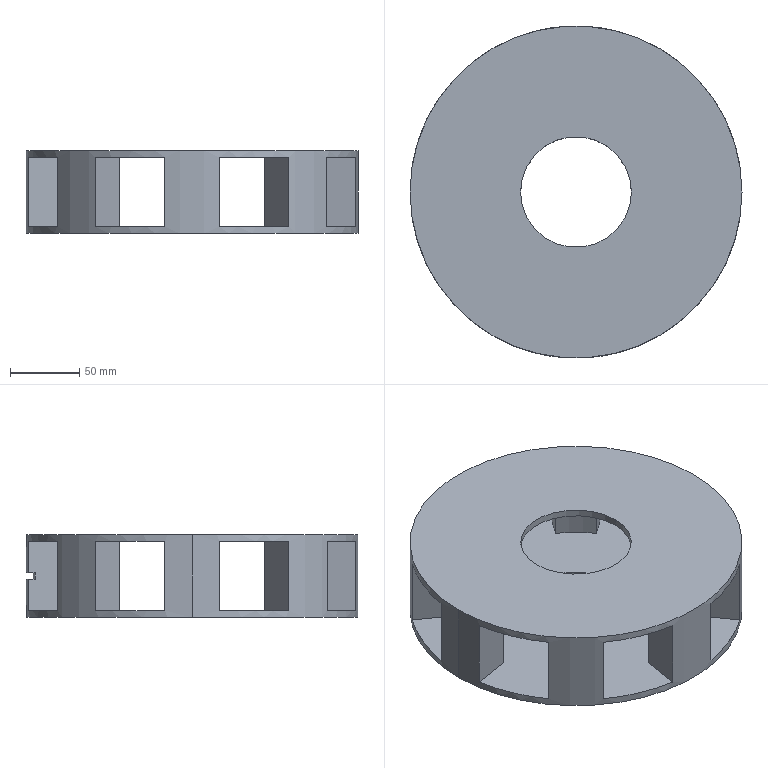Part | SolidWorks | features ICE 6, CirPattern 2, Extrusion 1, RevCut 1 | 1 solid | 38 faces | box 240 x 240 x 59.97 mm | volume 814702 mm3 | plane 22 | cylinder 16 | commonest cylinder face diameters 180 x9 80.06 x4 240 x2 230 x1
STEP:
#1=CARTESIAN_POINT('',(40.03,0.,5.));
#2=VERTEX_POINT('',#1);
#3=CARTESIAN_POINT('',(-40.03,0.,5.));
#4=VERTEX_POINT('',#3);
#5=CARTESIAN_POINT('',(0.,0.,5.));
#6=DIRECTION('',(0.,0.,-1.));
#7=DIRECTION('',(-1.,0.,0.));
#8=AXIS2_PLACEMENT_3D('',#5,#6,#7);
#9=CIRCLE('',#8,40.03);
#10=EDGE_CURVE('',#2,#4,#9,.T.);
#11=ORIENTED_EDGE('',*,*,#10,.F.);
#12=CARTESIAN_POINT('',(40.03,0.,0.));
#13=VERTEX_POINT('',#12);
#14=CARTESIAN_POINT('',(40.03,0.,5.));
#15=DIRECTION('',(0.,0.,-1.));
#16=VECTOR('',#15,1000.);
#17=LINE('',#14,#16);
#18=EDGE_CURVE('',#2,#13,#17,.T.);
#19=ORIENTED_EDGE('',*,*,#18,.T.);
#20=CARTESIAN_POINT('',(-40.03,0.,0.));
#21=VERTEX_POINT('',#20);
#22=CARTESIAN_POINT('',(0.,0.,0.));
#23=DIRECTION('',(0.,0.,-1.));
#24=DIRECTION('',(-1.,0.,0.));
#25=AXIS2_PLACEMENT_3D('',#22,#23,#24);
#26=CIRCLE('',#25,40.03);
#27=EDGE_CURVE('',#13,#21,#26,.T.);
#28=ORIENTED_EDGE('',*,*,#27,.T.);
#29=CARTESIAN_POINT('',(-40.03,0.,5.));
#30=DIRECTION('',(0.,0.,-1.));
#31=VECTOR('',#30,1000.);
#32=LINE('',#29,#31);
#33=EDGE_CURVE('',#4,#21,#32,.T.);
#34=ORIENTED_EDGE('',*,*,#33,.F.);
#35=EDGE_LOOP('',(#11,#19,#28,#34));
#36=FACE_OUTER_BOUND('',#35,.T.);
#37=CARTESIAN_POINT('',(0.,0.,5.));
#38=DIRECTION('',(0.,0.,-1.));
#39=DIRECTION('',(-1.,0.,0.));
#40=AXIS2_PLACEMENT_3D('',#37,#38,#39);
#41=CYLINDRICAL_SURFACE('',#40,40.03);
#42=ADVANCED_FACE('',(#36),#41,.F.);
#43=CARTESIAN_POINT('',(-40.03,0.,54.97));
#44=VERTEX_POINT('',#43);
#45=CARTESIAN_POINT('',(40.03,0.,54.97));
#46=VERTEX_POINT('',#45);
#47=CARTESIAN_POINT('',(0.,0.,54.97));
#48=DIRECTION('',(0.,0.,1.));
#49=DIRECTION('',(1.,0.,0.));
#50=AXIS2_PLACEMENT_3D('',#47,#48,#49);
#51=CIRCLE('',#50,40.03);
#52=EDGE_CURVE('',#44,#46,#51,.T.);
#53=ORIENTED_EDGE('',*,*,#52,.F.);
#54=CARTESIAN_POINT('',(-40.03,0.,59.97));
#55=VERTEX_POINT('',#54);
#56=CARTESIAN_POINT('',(-40.03,0.,54.97));
#57=DIRECTION('',(0.,0.,1.));
#58=VECTOR('',#57,1000.);
#59=LINE('',#56,#58);
#60=EDGE_CURVE('',#44,#55,#59,.T.);
#61=ORIENTED_EDGE('',*,*,#60,.T.);
#62=CARTESIAN_POINT('',(40.03,0.,59.97));
#63=VERTEX_POINT('',#62);
#64=CARTESIAN_POINT('',(0.,0.,59.97));
#65=DIRECTION('',(0.,0.,1.));
#66=DIRECTION('',(1.,0.,0.));
#67=AXIS2_PLACEMENT_3D('',#64,#65,#66);
#68=CIRCLE('',#67,40.03);
#69=EDGE_CURVE('',#55,#63,#68,.T.);
#70=ORIENTED_EDGE('',*,*,#69,.T.);
#71=CARTESIAN_POINT('',(40.03,0.,54.97));
#72=DIRECTION('',(0.,0.,1.));
#73=VECTOR('',#72,1000.);
#74=LINE('',#71,#73);
#75=EDGE_CURVE('',#46,#63,#74,.T.);
#76=ORIENTED_EDGE('',*,*,#75,.F.);
#77=EDGE_LOOP('',(#53,#61,#70,#76));
#78=FACE_OUTER_BOUND('',#77,.T.);
#79=CARTESIAN_POINT('',(0.,0.,54.97));
#80=DIRECTION('',(0.,0.,1.));
#81=DIRECTION('',(1.,0.,0.));
#82=AXIS2_PLACEMENT_3D('',#79,#80,#81);
#83=CYLINDRICAL_SURFACE('',#82,40.03);
#84=ADVANCED_FACE('',(#78),#83,.F.);
#85=CARTESIAN_POINT('',(-19.619,118.385,5.));
#86=VERTEX_POINT('',#85);
#87=CARTESIAN_POINT('',(-19.619,118.385,27.485));
#88=VERTEX_POINT('',#87);
#89=CARTESIAN_POINT('',(-19.619,118.385,80.));
#90=DIRECTION('',(0.,0.,1.));
#91=VECTOR('',#90,1000.);
#92=LINE('',#89,#91);
#93=EDGE_CURVE('',#86,#88,#92,.T.);
#94=ORIENTED_EDGE('',*,*,#93,.T.);
#95=CARTESIAN_POINT('',(19.619,118.385,27.485));
#96=VERTEX_POINT('',#95);
#97=CARTESIAN_POINT('',(0.,0.,27.485));
#98=DIRECTION('',(0.,0.,-1.));
#99=DIRECTION('',(-1.,0.,0.));
#100=AXIS2_PLACEMENT_3D('',#97,#98,#99);
#101=CIRCLE('',#100,120.);
#102=EDGE_CURVE('',#88,#96,#101,.T.);
#103=ORIENTED_EDGE('',*,*,#102,.T.);
#104=CARTESIAN_POINT('',(19.619,118.385,5.));
#105=VERTEX_POINT('',#104);
#106=CARTESIAN_POINT('',(19.619,118.385,80.));
#107=DIRECTION('',(0.,0.,-1.));
#108=VECTOR('',#107,1000.);
#109=LINE('',#106,#108);
#110=EDGE_CURVE('',#96,#105,#109,.T.);
#111=ORIENTED_EDGE('',*,*,#110,.T.);
#112=CARTESIAN_POINT('',(69.838,97.584,5.));
#113=VERTEX_POINT('',#112);
#114=CARTESIAN_POINT('',(0.,0.,5.));
#115=DIRECTION('',(0.,0.,-1.));
#116=DIRECTION('',(-1.,0.,0.));
#117=AXIS2_PLACEMENT_3D('',#114,#115,#116);
#118=CIRCLE('',#117,120.);
#119=EDGE_CURVE('',#105,#113,#118,.T.);
#120=ORIENTED_EDGE('',*,*,#119,.T.);
#121=CARTESIAN_POINT('',(69.838,97.584,54.97));
#122=VERTEX_POINT('',#121);
#123=CARTESIAN_POINT('',(69.838,97.584,80.));
#124=DIRECTION('',(0.,0.,1.));
#125=VECTOR('',#124,1000.);
#126=LINE('',#123,#125);
#127=EDGE_CURVE('',#113,#122,#126,.T.);
#128=ORIENTED_EDGE('',*,*,#127,.T.);
#129=CARTESIAN_POINT('',(19.619,118.385,54.97));
#130=VERTEX_POINT('',#129);
#131=CARTESIAN_POINT('',(0.,0.,54.97));
#132=DIRECTION('',(0.,0.,-1.));
#133=DIRECTION('',(-1.,0.,0.));
#134=AXIS2_PLACEMENT_3D('',#131,#132,#133);
#135=CIRCLE('',#134,120.);
#136=EDGE_CURVE('',#130,#122,#135,.T.);
#137=ORIENTED_EDGE('',*,*,#136,.F.);
#138=CARTESIAN_POINT('',(19.619,118.385,32.485));
#139=VERTEX_POINT('',#138);
#140=CARTESIAN_POINT('',(19.619,118.385,80.));
#141=DIRECTION('',(0.,0.,-1.));
#142=VECTOR('',#141,1000.);
#143=LINE('',#140,#142);
#144=EDGE_CURVE('',#130,#139,#143,.T.);
#145=ORIENTED_EDGE('',*,*,#144,.T.);
#146=CARTESIAN_POINT('',(-19.619,118.385,32.485));
#147=VERTEX_POINT('',#146);
#148=CARTESIAN_POINT('',(0.,0.,32.485));
#149=DIRECTION('',(0.,0.,1.));
#150=DIRECTION('',(1.,0.,0.));
#151=AXIS2_PLACEMENT_3D('',#148,#149,#150);
#152=CIRCLE('',#151,120.);
#153=EDGE_CURVE('',#139,#147,#152,.T.);
#154=ORIENTED_EDGE('',*,*,#153,.T.);
#155=CARTESIAN_POINT('',(-19.619,118.385,54.97));
#156=VERTEX_POINT('',#155);
#157=CARTESIAN_POINT('',(-19.619,118.385,80.));
#158=DIRECTION('',(0.,0.,1.));
#159=VECTOR('',#158,1000.);
#160=LINE('',#157,#159);
#161=EDGE_CURVE('',#147,#156,#160,.T.);
#162=ORIENTED_EDGE('',*,*,#161,.T.);
#163=CARTESIAN_POINT('',(-69.838,97.584,54.97));
#164=VERTEX_POINT('',#163);
#165=CARTESIAN_POINT('',(0.,0.,54.97));
#166=DIRECTION('',(0.,0.,-1.));
#167=DIRECTION('',(-1.,0.,0.));
#168=AXIS2_PLACEMENT_3D('',#165,#166,#167);
#169=CIRCLE('',#168,120.);
#170=EDGE_CURVE('',#164,#156,#169,.T.);
#171=ORIENTED_EDGE('',*,*,#170,.F.);
#172=CARTESIAN_POINT('',(-69.838,97.584,5.));
#173=VERTEX_POINT('',#172);
#174=CARTESIAN_POINT('',(-69.838,97.584,80.));
#175=DIRECTION('',(0.,0.,-1.));
#176=VECTOR('',#175,1000.);
#177=LINE('',#174,#176);
#178=EDGE_CURVE('',#164,#173,#177,.T.);
#179=ORIENTED_EDGE('',*,*,#178,.T.);
#180=CARTESIAN_POINT('',(0.,0.,5.));
#181=DIRECTION('',(0.,0.,-1.));
#182=DIRECTION('',(-1.,0.,0.));
#183=AXIS2_PLACEMENT_3D('',#180,#181,#182);
#184=CIRCLE('',#183,120.);
#185=EDGE_CURVE('',#173,#86,#184,.T.);
#186=ORIENTED_EDGE('',*,*,#185,.T.);
#187=EDGE_LOOP('',(#94,#103,#111,#120,#128,#137,#145,#154,#162,#171,#179,#186));
#188=FACE_BOUND('',#187,.T.);
#189=CARTESIAN_POINT('',(97.584,69.838,54.97));
#190=VERTEX_POINT('',#189);
#191=CARTESIAN_POINT('',(97.584,69.838,5.));
#192=VERTEX_POINT('',#191);
#193=CARTESIAN_POINT('',(97.584,69.838,80.));
#194=DIRECTION('',(0.,0.,-1.));
#195=VECTOR('',#194,1000.);
#196=LINE('',#193,#195);
#197=EDGE_CURVE('',#190,#192,#196,.T.);
#198=ORIENTED_EDGE('',*,*,#197,.T.);
#199=CARTESIAN_POINT('',(118.385,19.619,5.));
#200=VERTEX_POINT('',#199);
#201=CARTESIAN_POINT('',(0.,0.,5.));
#202=DIRECTION('',(0.,0.,-1.));
#203=DIRECTION('',(-1.,0.,0.));
#204=AXIS2_PLACEMENT_3D('',#201,#202,#203);
#205=CIRCLE('',#204,120.);
#206=EDGE_CURVE('',#192,#200,#205,.T.);
#207=ORIENTED_EDGE('',*,*,#206,.T.);
#208=CARTESIAN_POINT('',(118.385,19.619,54.97));
#209=VERTEX_POINT('',#208);
#210=CARTESIAN_POINT('',(118.385,19.619,80.));
#211=DIRECTION('',(0.,0.,1.));
#212=VECTOR('',#211,1000.);
#213=LINE('',#210,#212);
#214=EDGE_CURVE('',#200,#209,#213,.T.);
#215=ORIENTED_EDGE('',*,*,#214,.T.);
#216=CARTESIAN_POINT('',(0.,0.,54.97));
#217=DIRECTION('',(0.,0.,-1.));
#218=DIRECTION('',(-1.,0.,0.));
#219=AXIS2_PLACEMENT_3D('',#216,#217,#218);
#220=CIRCLE('',#219,120.);
#221=EDGE_CURVE('',#190,#209,#220,.T.);
#222=ORIENTED_EDGE('',*,*,#221,.F.);
#223=EDGE_LOOP('',(#198,#207,#215,#222));
#224=FACE_BOUND('',#223,.T.);
#225=CARTESIAN_POINT('',(-118.385,19.619,54.97));
#226=VERTEX_POINT('',#225);
#227=CARTESIAN_POINT('',(-118.385,19.619,5.));
#228=VERTEX_POINT('',#227);
#229=CARTESIAN_POINT('',(-118.385,19.619,80.));
#230=DIRECTION('',(0.,0.,-1.));
#231=VECTOR('',#230,1000.);
#232=LINE('',#229,#231);
#233=EDGE_CURVE('',#226,#228,#232,.T.);
#234=ORIENTED_EDGE('',*,*,#233,.T.);
#235=CARTESIAN_POINT('',(-97.584,69.838,5.));
#236=VERTEX_POINT('',#235);
#237=CARTESIAN_POINT('',(0.,0.,5.));
#238=DIRECTION('',(0.,0.,-1.));
#239=DIRECTION('',(-1.,0.,0.));
#240=AXIS2_PLACEMENT_3D('',#237,#238,#239);
#241=CIRCLE('',#240,120.);
#242=EDGE_CURVE('',#228,#236,#241,.T.);
#243=ORIENTED_EDGE('',*,*,#242,.T.);
#244=CARTESIAN_POINT('',(-97.584,69.838,54.97));
#245=VERTEX_POINT('',#244);
#246=CARTESIAN_POINT('',(-97.584,69.838,80.));
#247=DIRECTION('',(0.,0.,1.));
#248=VECTOR('',#247,1000.);
#249=LINE('',#246,#248);
#250=EDGE_CURVE('',#236,#245,#249,.T.);
#251=ORIENTED_EDGE('',*,*,#250,.T.);
#252=CARTESIAN_POINT('',(0.,0.,54.97));
#253=DIRECTION('',(0.,0.,-1.));
#254=DIRECTION('',(-1.,0.,0.));
#255=AXIS2_PLACEMENT_3D('',#252,#253,#254);
#256=CIRCLE('',#255,120.);
#257=EDGE_CURVE('',#226,#245,#256,.T.);
#258=ORIENTED_EDGE('',*,*,#257,.F.);
#259=EDGE_LOOP('',(#234,#243,#251,#258));
#260=FACE_BOUND('',#259,.T.);
#261=CARTESIAN_POINT('',(-120.,0.,0.));
#262=VERTEX_POINT('',#261);
#263=CARTESIAN_POINT('',(120.,0.,0.));
#264=VERTEX_POINT('',#263);
#265=CARTESIAN_POINT('',(0.,0.,0.));
#266=DIRECTION('',(0.,0.,-1.));
#267=DIRECTION('',(1.,0.,0.));
#268=AXIS2_PLACEMENT_3D('',#265,#266,#267);
#269=CIRCLE('',#268,120.);
#270=EDGE_CURVE('',#262,#264,#269,.T.);
#271=ORIENTED_EDGE('',*,*,#270,.F.);
#272=CARTESIAN_POINT('',(-120.,0.,59.97));
#273=VERTEX_POINT('',#272);
#274=CARTESIAN_POINT('',(-120.,0.,0.));
#275=DIRECTION('',(0.,0.,1.));
#276=VECTOR('',#275,1000.);
#277=LINE('',#274,#276);
#278=EDGE_CURVE('',#262,#273,#277,.T.);
#279=ORIENTED_EDGE('',*,*,#278,.T.);
#280=CARTESIAN_POINT('',(120.,0.,59.97));
#281=VERTEX_POINT('',#280);
#282=CARTESIAN_POINT('',(0.,0.,59.97));
#283=DIRECTION('',(0.,0.,-1.));
#284=DIRECTION('',(1.,0.,0.));
#285=AXIS2_PLACEMENT_3D('',#282,#283,#284);
#286=CIRCLE('',#285,120.);
#287=EDGE_CURVE('',#273,#281,#286,.T.);
#288=ORIENTED_EDGE('',*,*,#287,.T.);
#289=CARTESIAN_POINT('',(120.,0.,0.));
#290=DIRECTION('',(0.,0.,1.));
#291=VECTOR('',#290,1000.);
#292=LINE('',#289,#291);
#293=EDGE_CURVE('',#264,#281,#292,.T.);
#294=ORIENTED_EDGE('',*,*,#293,.F.);
#295=EDGE_LOOP('',(#271,#279,#288,#294));
#296=FACE_OUTER_BOUND('',#295,.T.);
#297=CARTESIAN_POINT('',(0.,0.,0.));
#298=DIRECTION('',(0.,0.,1.));
#299=DIRECTION('',(1.,0.,0.));
#300=AXIS2_PLACEMENT_3D('',#297,#298,#299);
#301=CYLINDRICAL_SURFACE('',#300,120.);
#302=ADVANCED_FACE('',(#188,#224,#260,#296),#301,.T.);
#303=CARTESIAN_POINT('',(88.789,14.715,5.));
#304=VERTEX_POINT('',#303);
#305=CARTESIAN_POINT('',(90.,0.,5.));
#306=VERTEX_POINT('',#305);
#307=CARTESIAN_POINT('',(0.,0.,5.));
#308=DIRECTION('',(0.,0.,-1.));
#309=DIRECTION('',(-1.,0.,0.));
#310=AXIS2_PLACEMENT_3D('',#307,#308,#309);
#311=CIRCLE('',#310,90.);
#312=EDGE_CURVE('',#304,#306,#311,.T.);
#313=ORIENTED_EDGE('',*,*,#312,.T.);
#314=CARTESIAN_POINT('',(90.,0.,54.97));
#315=VERTEX_POINT('',#314);
#316=CARTESIAN_POINT('',(90.,0.,0.));
#317=DIRECTION('',(0.,0.,1.));
#318=VECTOR('',#317,1000.);
#319=LINE('',#316,#318);
#320=EDGE_CURVE('',#306,#315,#319,.T.);
#321=ORIENTED_EDGE('',*,*,#320,.T.);
#322=CARTESIAN_POINT('',(88.789,14.715,54.97));
#323=VERTEX_POINT('',#322);
#324=CARTESIAN_POINT('',(0.,0.,54.97));
#325=DIRECTION('',(0.,0.,1.));
#326=DIRECTION('',(1.,0.,0.));
#327=AXIS2_PLACEMENT_3D('',#324,#325,#326);
#328=CIRCLE('',#327,90.);
#329=EDGE_CURVE('',#315,#323,#328,.T.);
#330=ORIENTED_EDGE('',*,*,#329,.T.);
#331=CARTESIAN_POINT('',(88.789,14.715,5.));
#332=DIRECTION('',(0.,0.,1.));
#333=VECTOR('',#332,1000.);
#334=LINE('',#331,#333);
#335=EDGE_CURVE('',#304,#323,#334,.T.);
#336=ORIENTED_EDGE('',*,*,#335,.F.);
#337=EDGE_LOOP('',(#313,#321,#330,#336));
#338=FACE_OUTER_BOUND('',#337,.T.);
#339=CARTESIAN_POINT('',(0.,0.,0.));
#340=DIRECTION('',(0.,0.,1.));
#341=DIRECTION('',(1.,0.,0.));
#342=AXIS2_PLACEMENT_3D('',#339,#340,#341);
#343=CYLINDRICAL_SURFACE('',#342,90.);
#344=ADVANCED_FACE('',(#338),#343,.F.);
#345=CARTESIAN_POINT('',(0.,0.,59.97));
#346=DIRECTION('',(0.,0.,1.));
#347=DIRECTION('',(1.,0.,0.));
#348=AXIS2_PLACEMENT_3D('',#345,#346,#347);
#349=CIRCLE('',#348,40.03);
#350=EDGE_CURVE('',#63,#55,#349,.T.);
#351=ORIENTED_EDGE('',*,*,#350,.F.);
#352=ORIENTED_EDGE('',*,*,#69,.F.);
#353=EDGE_LOOP('',(#351,#352));
#354=FACE_BOUND('',#353,.T.);
#355=CARTESIAN_POINT('',(0.,0.,59.97));
#356=DIRECTION('',(0.,0.,-1.));
#357=DIRECTION('',(1.,0.,0.));
#358=AXIS2_PLACEMENT_3D('',#355,#356,#357);
#359=CIRCLE('',#358,120.);
#360=EDGE_CURVE('',#281,#273,#359,.T.);
#361=ORIENTED_EDGE('',*,*,#360,.F.);
#362=ORIENTED_EDGE('',*,*,#287,.F.);
#363=EDGE_LOOP('',(#361,#362));
#364=FACE_OUTER_BOUND('',#363,.T.);
#365=CARTESIAN_POINT('',(0.,0.,59.97));
#366=DIRECTION('',(0.,0.,1.));
#367=DIRECTION('',(1.,0.,0.));
#368=AXIS2_PLACEMENT_3D('',#365,#366,#367);
#369=PLANE('',#368);
#370=ADVANCED_FACE('',(#354,#364),#369,.T.);
#371=CARTESIAN_POINT('',(0.,0.,0.));
#372=DIRECTION('',(0.,0.,-1.));
#373=DIRECTION('',(-1.,0.,0.));
#374=AXIS2_PLACEMENT_3D('',#371,#372,#373);
#375=CIRCLE('',#374,40.03);
#376=EDGE_CURVE('',#21,#13,#375,.T.);
#377=ORIENTED_EDGE('',*,*,#376,.F.);
#378=ORIENTED_EDGE('',*,*,#27,.F.);
#379=EDGE_LOOP('',(#377,#378));
#380=FACE_BOUND('',#379,.T.);
#381=CARTESIAN_POINT('',(0.,0.,0.));
#382=DIRECTION('',(0.,0.,-1.));
#383=DIRECTION('',(1.,0.,0.));
#384=AXIS2_PLACEMENT_3D('',#381,#382,#383);
#385=CIRCLE('',#384,120.);
#386=EDGE_CURVE('',#264,#262,#385,.T.);
#387=ORIENTED_EDGE('',*,*,#386,.T.);
#388=ORIENTED_EDGE('',*,*,#270,.T.);
#389=EDGE_LOOP('',(#387,#388));
#390=FACE_OUTER_BOUND('',#389,.T.);
#391=CARTESIAN_POINT('',(0.,0.,0.));
#392=DIRECTION('',(0.,0.,1.));
#393=DIRECTION('',(1.,0.,0.));
#394=AXIS2_PLACEMENT_3D('',#391,#392,#393);
#395=PLANE('',#394);
#396=ADVANCED_FACE('',(#380,#390),#395,.F.);
#397=ORIENTED_EDGE('',*,*,#110,.F.);
#398=CARTESIAN_POINT('',(18.802,113.453,27.485));
#399=VERTEX_POINT('',#398);
#400=CARTESIAN_POINT('',(19.619,118.385,27.485));
#401=DIRECTION('',(0.1635,0.9865,0.));
#402=VECTOR('',#401,1000.);
#403=LINE('',#400,#402);
#404=EDGE_CURVE('',#399,#96,#403,.T.);
#405=ORIENTED_EDGE('',*,*,#404,.F.);
#406=CARTESIAN_POINT('',(18.802,113.453,32.485));
#407=VERTEX_POINT('',#406);
#408=CARTESIAN_POINT('',(18.802,113.453,32.485));
#409=DIRECTION('',(0.,0.,-1.));
#410=VECTOR('',#409,1000.);
#411=LINE('',#408,#410);
#412=EDGE_CURVE('',#407,#399,#411,.T.);
#413=ORIENTED_EDGE('',*,*,#412,.F.);
#414=CARTESIAN_POINT('',(19.619,118.385,32.485));
#415=DIRECTION('',(-0.1635,-0.9865,0.));
#416=VECTOR('',#415,1000.);
#417=LINE('',#414,#416);
#418=EDGE_CURVE('',#139,#407,#417,.T.);
#419=ORIENTED_EDGE('',*,*,#418,.F.);
#420=ORIENTED_EDGE('',*,*,#144,.F.);
#421=CARTESIAN_POINT('',(14.715,88.789,54.97));
#422=VERTEX_POINT('',#421);
#423=CARTESIAN_POINT('',(14.715,88.789,54.97));
#424=DIRECTION('',(-0.1635,-0.9865,0.));
#425=VECTOR('',#424,1000.);
#426=LINE('',#423,#425);
#427=EDGE_CURVE('',#130,#422,#426,.T.);
#428=ORIENTED_EDGE('',*,*,#427,.T.);
#429=CARTESIAN_POINT('',(14.715,88.789,5.));
#430=VERTEX_POINT('',#429);
#431=CARTESIAN_POINT('',(14.715,88.789,5.));
#432=DIRECTION('',(0.,0.,1.));
#433=VECTOR('',#432,1000.);
#434=LINE('',#431,#433);
#435=EDGE_CURVE('',#430,#422,#434,.T.);
#436=ORIENTED_EDGE('',*,*,#435,.F.);
#437=CARTESIAN_POINT('',(14.715,88.789,5.));
#438=DIRECTION('',(-0.1635,-0.9865,0.));
#439=VECTOR('',#438,1000.);
#440=LINE('',#437,#439);
#441=EDGE_CURVE('',#105,#430,#440,.T.);
#442=ORIENTED_EDGE('',*,*,#441,.F.);
#443=EDGE_LOOP('',(#397,#405,#413,#419,#420,#428,#436,#442));
#444=FACE_OUTER_BOUND('',#443,.T.);
#445=CARTESIAN_POINT('',(14.715,88.789,5.));
#446=DIRECTION('',(-0.9865,0.1635,0.));
#447=DIRECTION('',(-0.1635,-0.9865,0.));
#448=AXIS2_PLACEMENT_3D('',#445,#446,#447);
#449=PLANE('',#448);
#450=ADVANCED_FACE('',(#444),#449,.F.);
#451=ORIENTED_EDGE('',*,*,#127,.F.);
#452=CARTESIAN_POINT('',(52.378,73.188,5.));
#453=VERTEX_POINT('',#452);
#454=CARTESIAN_POINT('',(52.378,73.188,5.));
#455=DIRECTION('',(0.582,0.8132,0.));
#456=VECTOR('',#455,1000.);
#457=LINE('',#454,#456);
#458=EDGE_CURVE('',#453,#113,#457,.T.);
#459=ORIENTED_EDGE('',*,*,#458,.F.);
#460=CARTESIAN_POINT('',(52.378,73.188,54.97));
#461=VERTEX_POINT('',#460);
#462=CARTESIAN_POINT('',(52.378,73.188,5.));
#463=DIRECTION('',(0.,0.,1.));
#464=VECTOR('',#463,1000.);
#465=LINE('',#462,#464);
#466=EDGE_CURVE('',#453,#461,#465,.T.);
#467=ORIENTED_EDGE('',*,*,#466,.T.);
#468=CARTESIAN_POINT('',(52.378,73.188,54.97));
#469=DIRECTION('',(0.582,0.8132,0.));
#470=VECTOR('',#469,1000.);
#471=LINE('',#468,#470);
#472=EDGE_CURVE('',#461,#122,#471,.T.);
#473=ORIENTED_EDGE('',*,*,#472,.T.);
#474=EDGE_LOOP('',(#451,#459,#467,#473));
#475=FACE_OUTER_BOUND('',#474,.T.);
#476=CARTESIAN_POINT('',(52.378,73.188,5.));
#477=DIRECTION('',(0.8132,-0.582,0.));
#478=DIRECTION('',(0.582,0.8132,0.));
#479=AXIS2_PLACEMENT_3D('',#476,#477,#478);
#480=PLANE('',#479);
#481=ADVANCED_FACE('',(#475),#480,.F.);
#482=CARTESIAN_POINT('',(0.,0.,5.));
#483=DIRECTION('',(0.,0.,-1.));
#484=DIRECTION('',(-1.,0.,0.));
#485=AXIS2_PLACEMENT_3D('',#482,#483,#484);
#486=CIRCLE('',#485,40.03);
#487=EDGE_CURVE('',#4,#2,#486,.T.);
#488=ORIENTED_EDGE('',*,*,#487,.T.);
#489=ORIENTED_EDGE('',*,*,#10,.T.);
#490=EDGE_LOOP('',(#488,#489));
#491=FACE_BOUND('',#490,.T.);
#492=ORIENTED_EDGE('',*,*,#242,.F.);
#493=CARTESIAN_POINT('',(-88.789,14.715,5.));
#494=VERTEX_POINT('',#493);
#495=CARTESIAN_POINT('',(-88.789,14.715,5.));
#496=DIRECTION('',(0.9865,-0.1635,0.));
#497=VECTOR('',#496,1000.);
#498=LINE('',#495,#497);
#499=EDGE_CURVE('',#228,#494,#498,.T.);
#500=ORIENTED_EDGE('',*,*,#499,.T.);
#501=CARTESIAN_POINT('',(-88.789,-14.715,5.));
#502=VERTEX_POINT('',#501);
#503=CARTESIAN_POINT('',(0.,0.,5.));
#504=DIRECTION('',(0.,0.,-1.));
#505=DIRECTION('',(-1.,0.,0.));
#506=AXIS2_PLACEMENT_3D('',#503,#504,#505);
#507=CIRCLE('',#506,90.);
#508=EDGE_CURVE('',#502,#494,#507,.T.);
#509=ORIENTED_EDGE('',*,*,#508,.F.);
#510=CARTESIAN_POINT('',(-118.385,-19.619,5.));
#511=VERTEX_POINT('',#510);
#512=CARTESIAN_POINT('',(-88.789,-14.715,5.));
#513=DIRECTION('',(-0.9865,-0.1635,0.));
#514=VECTOR('',#513,1000.);
#515=LINE('',#512,#514);
#516=EDGE_CURVE('',#502,#511,#515,.T.);
#517=ORIENTED_EDGE('',*,*,#516,.T.);
#518=CARTESIAN_POINT('',(-97.584,-69.838,5.));
#519=VERTEX_POINT('',#518);
#520=CARTESIAN_POINT('',(0.,0.,5.));
#521=DIRECTION('',(0.,0.,-1.));
#522=DIRECTION('',(-1.,0.,0.));
#523=AXIS2_PLACEMENT_3D('',#520,#521,#522);
#524=CIRCLE('',#523,120.);
#525=EDGE_CURVE('',#519,#511,#524,.T.);
#526=ORIENTED_EDGE('',*,*,#525,.F.);
#527=CARTESIAN_POINT('',(-73.188,-52.378,5.));
#528=VERTEX_POINT('',#527);
#529=CARTESIAN_POINT('',(-73.188,-52.378,5.));
#530=DIRECTION('',(0.8132,0.582,0.));
#531=VECTOR('',#530,1000.);
#532=LINE('',#529,#531);
#533=EDGE_CURVE('',#519,#528,#532,.T.);
#534=ORIENTED_EDGE('',*,*,#533,.T.);
#535=CARTESIAN_POINT('',(-52.378,-73.188,5.));
#536=VERTEX_POINT('',#535);
#537=CARTESIAN_POINT('',(0.,0.,5.));
#538=DIRECTION('',(0.,0.,-1.));
#539=DIRECTION('',(-1.,0.,0.));
#540=AXIS2_PLACEMENT_3D('',#537,#538,#539);
#541=CIRCLE('',#540,90.);
#542=EDGE_CURVE('',#536,#528,#541,.T.);
#543=ORIENTED_EDGE('',*,*,#542,.F.);
#544=CARTESIAN_POINT('',(-69.838,-97.584,5.));
#545=VERTEX_POINT('',#544);
#546=CARTESIAN_POINT('',(-52.378,-73.188,5.));
#547=DIRECTION('',(-0.582,-0.8132,0.));
#548=VECTOR('',#547,1000.);
#549=LINE('',#546,#548);
#550=EDGE_CURVE('',#536,#545,#549,.T.);
#551=ORIENTED_EDGE('',*,*,#550,.T.);
#552=CARTESIAN_POINT('',(-19.619,-118.385,5.));
#553=VERTEX_POINT('',#552);
#554=CARTESIAN_POINT('',(0.,0.,5.));
#555=DIRECTION('',(0.,0.,-1.));
#556=DIRECTION('',(-1.,0.,0.));
#557=AXIS2_PLACEMENT_3D('',#554,#555,#556);
#558=CIRCLE('',#557,120.);
#559=EDGE_CURVE('',#553,#545,#558,.T.);
#560=ORIENTED_EDGE('',*,*,#559,.F.);
#561=CARTESIAN_POINT('',(-14.715,-88.789,5.));
#562=VERTEX_POINT('',#561);
#563=CARTESIAN_POINT('',(-14.715,-88.789,5.));
#564=DIRECTION('',(0.1635,0.9865,0.));
#565=VECTOR('',#564,1000.);
#566=LINE('',#563,#565);
#567=EDGE_CURVE('',#553,#562,#566,.T.);
#568=ORIENTED_EDGE('',*,*,#567,.T.);
#569=CARTESIAN_POINT('',(14.715,-88.789,5.));
#570=VERTEX_POINT('',#569);
#571=CARTESIAN_POINT('',(0.,0.,5.));
#572=DIRECTION('',(0.,0.,-1.));
#573=DIRECTION('',(-1.,0.,0.));
#574=AXIS2_PLACEMENT_3D('',#571,#572,#573);
#575=CIRCLE('',#574,90.);
#576=EDGE_CURVE('',#570,#562,#575,.T.);
#577=ORIENTED_EDGE('',*,*,#576,.F.);
#578=CARTESIAN_POINT('',(19.619,-118.385,5.));
#579=VERTEX_POINT('',#578);
#580=CARTESIAN_POINT('',(14.715,-88.789,5.));
#581=DIRECTION('',(0.1635,-0.9865,0.));
#582=VECTOR('',#581,1000.);
#583=LINE('',#580,#582);
#584=EDGE_CURVE('',#570,#579,#583,.T.);
#585=ORIENTED_EDGE('',*,*,#584,.T.);
#586=CARTESIAN_POINT('',(69.838,-97.584,5.));
#587=VERTEX_POINT('',#586);
#588=CARTESIAN_POINT('',(0.,0.,5.));
#589=DIRECTION('',(0.,0.,-1.));
#590=DIRECTION('',(-1.,0.,0.));
#591=AXIS2_PLACEMENT_3D('',#588,#589,#590);
#592=CIRCLE('',#591,120.);
#593=EDGE_CURVE('',#587,#579,#592,.T.);
#594=ORIENTED_EDGE('',*,*,#593,.F.);
#595=CARTESIAN_POINT('',(52.378,-73.188,5.));
#596=VERTEX_POINT('',#595);
#597=CARTESIAN_POINT('',(52.378,-73.188,5.));
#598=DIRECTION('',(-0.582,0.8132,0.));
#599=VECTOR('',#598,1000.);
#600=LINE('',#597,#599);
#601=EDGE_CURVE('',#587,#596,#600,.T.);
#602=ORIENTED_EDGE('',*,*,#601,.T.);
#603=CARTESIAN_POINT('',(73.188,-52.378,5.));
#604=VERTEX_POINT('',#603);
#605=CARTESIAN_POINT('',(0.,0.,5.));
#606=DIRECTION('',(0.,0.,-1.));
#607=DIRECTION('',(-1.,0.,0.));
#608=AXIS2_PLACEMENT_3D('',#605,#606,#607);
#609=CIRCLE('',#608,90.);
#610=EDGE_CURVE('',#604,#596,#609,.T.);
#611=ORIENTED_EDGE('',*,*,#610,.F.);
#612=CARTESIAN_POINT('',(97.584,-69.838,5.));
#613=VERTEX_POINT('',#612);
#614=CARTESIAN_POINT('',(73.188,-52.378,5.));
#615=DIRECTION('',(0.8132,-0.582,0.));
#616=VECTOR('',#615,1000.);
#617=LINE('',#614,#616);
#618=EDGE_CURVE('',#604,#613,#617,.T.);
#619=ORIENTED_EDGE('',*,*,#618,.T.);
#620=CARTESIAN_POINT('',(118.385,-19.619,5.));
#621=VERTEX_POINT('',#620);
#622=CARTESIAN_POINT('',(0.,0.,5.));
#623=DIRECTION('',(0.,0.,-1.));
#624=DIRECTION('',(-1.,0.,0.));
#625=AXIS2_PLACEMENT_3D('',#622,#623,#624);
#626=CIRCLE('',#625,120.);
#627=EDGE_CURVE('',#621,#613,#626,.T.);
#628=ORIENTED_EDGE('',*,*,#627,.F.);
#629=CARTESIAN_POINT('',(88.789,-14.715,5.));
#630=VERTEX_POINT('',#629);
#631=CARTESIAN_POINT('',(88.789,-14.715,5.));
#632=DIRECTION('',(-0.9865,0.1635,0.));
#633=VECTOR('',#632,1000.);
#634=LINE('',#631,#633);
#635=EDGE_CURVE('',#621,#630,#634,.T.);
#636=ORIENTED_EDGE('',*,*,#635,.T.);
#637=CARTESIAN_POINT('',(0.,0.,5.));
#638=DIRECTION('',(0.,0.,-1.));
#639=DIRECTION('',(-1.,0.,0.));
#640=AXIS2_PLACEMENT_3D('',#637,#638,#639);
#641=CIRCLE('',#640,90.);
#642=EDGE_CURVE('',#306,#630,#641,.T.);
#643=ORIENTED_EDGE('',*,*,#642,.F.);
#644=ORIENTED_EDGE('',*,*,#312,.F.);
#645=CARTESIAN_POINT('',(88.789,14.715,5.));
#646=DIRECTION('',(0.9865,0.1635,0.));
#647=VECTOR('',#646,1000.);
#648=LINE('',#645,#647);
#649=EDGE_CURVE('',#304,#200,#648,.T.);
#650=ORIENTED_EDGE('',*,*,#649,.T.);
#651=ORIENTED_EDGE('',*,*,#206,.F.);
#652=CARTESIAN_POINT('',(73.188,52.378,5.));
#653=VERTEX_POINT('',#652);
#654=CARTESIAN_POINT('',(73.188,52.378,5.));
#655=DIRECTION('',(-0.8132,-0.582,0.));
#656=VECTOR('',#655,1000.);
#657=LINE('',#654,#656);
#658=EDGE_CURVE('',#192,#653,#657,.T.);
#659=ORIENTED_EDGE('',*,*,#658,.T.);
#660=CARTESIAN_POINT('',(0.,0.,5.));
#661=DIRECTION('',(0.,0.,-1.));
#662=DIRECTION('',(-1.,0.,0.));
#663=AXIS2_PLACEMENT_3D('',#660,#661,#662);
#664=CIRCLE('',#663,90.);
#665=EDGE_CURVE('',#453,#653,#664,.T.);
#666=ORIENTED_EDGE('',*,*,#665,.F.);
#667=ORIENTED_EDGE('',*,*,#458,.T.);
#668=ORIENTED_EDGE('',*,*,#119,.F.);
#669=ORIENTED_EDGE('',*,*,#441,.T.);
#670=CARTESIAN_POINT('',(-14.715,88.789,5.));
#671=VERTEX_POINT('',#670);
#672=CARTESIAN_POINT('',(0.,0.,5.));
#673=DIRECTION('',(0.,0.,-1.));
#674=DIRECTION('',(-1.,0.,0.));
#675=AXIS2_PLACEMENT_3D('',#672,#673,#674);
#676=CIRCLE('',#675,90.);
#677=EDGE_CURVE('',#671,#430,#676,.T.);
#678=ORIENTED_EDGE('',*,*,#677,.F.);
#679=CARTESIAN_POINT('',(-14.715,88.789,5.));
#680=DIRECTION('',(-0.1635,0.9865,0.));
#681=VECTOR('',#680,1000.);
#682=LINE('',#679,#681);
#683=EDGE_CURVE('',#671,#86,#682,.T.);
#684=ORIENTED_EDGE('',*,*,#683,.T.);
#685=ORIENTED_EDGE('',*,*,#185,.F.);
#686=CARTESIAN_POINT('',(-52.378,73.188,5.));
#687=VERTEX_POINT('',#686);
#688=CARTESIAN_POINT('',(-52.378,73.188,5.));
#689=DIRECTION('',(0.582,-0.8132,0.));
#690=VECTOR('',#689,1000.);
#691=LINE('',#688,#690);
#692=EDGE_CURVE('',#173,#687,#691,.T.);
#693=ORIENTED_EDGE('',*,*,#692,.T.);
#694=CARTESIAN_POINT('',(-73.188,52.378,5.));
#695=VERTEX_POINT('',#694);
#696=CARTESIAN_POINT('',(0.,0.,5.));
#697=DIRECTION('',(0.,0.,-1.));
#698=DIRECTION('',(-1.,0.,0.));
#699=AXIS2_PLACEMENT_3D('',#696,#697,#698);
#700=CIRCLE('',#699,90.);
#701=EDGE_CURVE('',#695,#687,#700,.T.);
#702=ORIENTED_EDGE('',*,*,#701,.F.);
#703=CARTESIAN_POINT('',(-73.188,52.378,5.));
#704=DIRECTION('',(-0.8132,0.582,0.));
#705=VECTOR('',#704,1000.);
#706=LINE('',#703,#705);
#707=EDGE_CURVE('',#695,#236,#706,.T.);
#708=ORIENTED_EDGE('',*,*,#707,.T.);
#709=EDGE_LOOP('',(#492,#500,#509,#517,#526,#534,#543,#551,#560,#568,#577,#585,#594,#602,#611,#619,#628,#636,#643,#644,#650,#651,#659,#666,#667,#668,#669,#678,#684,#685,#693,#702,#708));
#710=FACE_OUTER_BOUND('',#709,.T.);
#711=CARTESIAN_POINT('',(0.,0.,5.));
#712=DIRECTION('',(0.,0.,-1.));
#713=DIRECTION('',(-1.,0.,0.));
#714=AXIS2_PLACEMENT_3D('',#711,#712,#713);
#715=PLANE('',#714);
#716=ADVANCED_FACE('',(#491,#710),#715,.F.);
#717=CARTESIAN_POINT('',(0.,0.,54.97));
#718=DIRECTION('',(0.,0.,1.));
#719=DIRECTION('',(1.,0.,0.));
#720=AXIS2_PLACEMENT_3D('',#717,#718,#719);
#721=CIRCLE('',#720,40.03);
#722=EDGE_CURVE('',#46,#44,#721,.T.);
#723=ORIENTED_EDGE('',*,*,#722,.T.);
#724=ORIENTED_EDGE('',*,*,#52,.T.);
#725=EDGE_LOOP('',(#723,#724));
#726=FACE_BOUND('',#725,.T.);
#727=CARTESIAN_POINT('',(-88.789,14.715,54.97));
#728=VERTEX_POINT('',#727);
#729=CARTESIAN_POINT('',(-88.789,14.715,54.97));
#730=DIRECTION('',(0.9865,-0.1635,0.));
#731=VECTOR('',#730,1000.);
#732=LINE('',#729,#731);
#733=EDGE_CURVE('',#226,#728,#732,.T.);
#734=ORIENTED_EDGE('',*,*,#733,.F.);
#735=ORIENTED_EDGE('',*,*,#257,.T.);
#736=CARTESIAN_POINT('',(-73.188,52.378,54.97));
#737=VERTEX_POINT('',#736);
#738=CARTESIAN_POINT('',(-73.188,52.378,54.97));
#739=DIRECTION('',(-0.8132,0.582,0.));
#740=VECTOR('',#739,1000.);
#741=LINE('',#738,#740);
#742=EDGE_CURVE('',#737,#245,#741,.T.);
#743=ORIENTED_EDGE('',*,*,#742,.F.);
#744=CARTESIAN_POINT('',(-52.378,73.188,54.97));
#745=VERTEX_POINT('',#744);
#746=CARTESIAN_POINT('',(0.,0.,54.97));
#747=DIRECTION('',(0.,0.,1.));
#748=DIRECTION('',(1.,0.,0.));
#749=AXIS2_PLACEMENT_3D('',#746,#747,#748);
#750=CIRCLE('',#749,90.);
#751=EDGE_CURVE('',#745,#737,#750,.T.);
#752=ORIENTED_EDGE('',*,*,#751,.F.);
#753=CARTESIAN_POINT('',(-52.378,73.188,54.97));
#754=DIRECTION('',(0.582,-0.8132,0.));
#755=VECTOR('',#754,1000.);
#756=LINE('',#753,#755);
#757=EDGE_CURVE('',#164,#745,#756,.T.);
#758=ORIENTED_EDGE('',*,*,#757,.F.);
#759=ORIENTED_EDGE('',*,*,#170,.T.);
#760=CARTESIAN_POINT('',(-14.715,88.789,54.97));
#761=VERTEX_POINT('',#760);
#762=CARTESIAN_POINT('',(-14.715,88.789,54.97));
#763=DIRECTION('',(-0.1635,0.9865,0.));
#764=VECTOR('',#763,1000.);
#765=LINE('',#762,#764);
#766=EDGE_CURVE('',#761,#156,#765,.T.);
#767=ORIENTED_EDGE('',*,*,#766,.F.);
#768=CARTESIAN_POINT('',(0.,0.,54.97));
#769=DIRECTION('',(0.,0.,1.));
#770=DIRECTION('',(1.,0.,0.));
#771=AXIS2_PLACEMENT_3D('',#768,#769,#770);
#772=CIRCLE('',#771,90.);
#773=EDGE_CURVE('',#422,#761,#772,.T.);
#774=ORIENTED_EDGE('',*,*,#773,.F.);
#775=ORIENTED_EDGE('',*,*,#427,.F.);
#776=ORIENTED_EDGE('',*,*,#136,.T.);
#777=ORIENTED_EDGE('',*,*,#472,.F.);
#778=CARTESIAN_POINT('',(73.188,52.378,54.97));
#779=VERTEX_POINT('',#778);
#780=CARTESIAN_POINT('',(0.,0.,54.97));
#781=DIRECTION('',(0.,0.,1.));
#782=DIRECTION('',(1.,0.,0.));
#783=AXIS2_PLACEMENT_3D('',#780,#781,#782);
#784=CIRCLE('',#783,90.);
#785=EDGE_CURVE('',#779,#461,#784,.T.);
#786=ORIENTED_EDGE('',*,*,#785,.F.);
#787=CARTESIAN_POINT('',(73.188,52.378,54.97));
#788=DIRECTION('',(-0.8132,-0.582,0.));
#789=VECTOR('',#788,1000.);
#790=LINE('',#787,#789);
#791=EDGE_CURVE('',#190,#779,#790,.T.);
#792=ORIENTED_EDGE('',*,*,#791,.F.);
#793=ORIENTED_EDGE('',*,*,#221,.T.);
#794=CARTESIAN_POINT('',(88.789,14.715,54.97));
#795=DIRECTION('',(0.9865,0.1635,0.));
#796=VECTOR('',#795,1000.);
#797=LINE('',#794,#796);
#798=EDGE_CURVE('',#323,#209,#797,.T.);
#799=ORIENTED_EDGE('',*,*,#798,.F.);
#800=ORIENTED_EDGE('',*,*,#329,.F.);
#801=CARTESIAN_POINT('',(88.789,-14.715,54.97));
#802=VERTEX_POINT('',#801);
#803=CARTESIAN_POINT('',(0.,0.,54.97));
#804=DIRECTION('',(0.,0.,1.));
#805=DIRECTION('',(1.,0.,0.));
#806=AXIS2_PLACEMENT_3D('',#803,#804,#805);
#807=CIRCLE('',#806,90.);
#808=EDGE_CURVE('',#802,#315,#807,.T.);
#809=ORIENTED_EDGE('',*,*,#808,.F.);
#810=CARTESIAN_POINT('',(118.385,-19.619,54.97));
#811=VERTEX_POINT('',#810);
#812=CARTESIAN_POINT('',(88.789,-14.715,54.97));
#813=DIRECTION('',(-0.9865,0.1635,0.));
#814=VECTOR('',#813,1000.);
#815=LINE('',#812,#814);
#816=EDGE_CURVE('',#811,#802,#815,.T.);
#817=ORIENTED_EDGE('',*,*,#816,.F.);
#818=CARTESIAN_POINT('',(97.584,-69.838,54.97));
#819=VERTEX_POINT('',#818);
#820=CARTESIAN_POINT('',(0.,0.,54.97));
#821=DIRECTION('',(0.,0.,-1.));
#822=DIRECTION('',(-1.,0.,0.));
#823=AXIS2_PLACEMENT_3D('',#820,#821,#822);
#824=CIRCLE('',#823,120.);
#825=EDGE_CURVE('',#811,#819,#824,.T.);
#826=ORIENTED_EDGE('',*,*,#825,.T.);
#827=CARTESIAN_POINT('',(73.188,-52.378,54.97));
#828=VERTEX_POINT('',#827);
#829=CARTESIAN_POINT('',(73.188,-52.378,54.97));
#830=DIRECTION('',(0.8132,-0.582,0.));
#831=VECTOR('',#830,1000.);
#832=LINE('',#829,#831);
#833=EDGE_CURVE('',#828,#819,#832,.T.);
#834=ORIENTED_EDGE('',*,*,#833,.F.);
#835=CARTESIAN_POINT('',(52.378,-73.188,54.97));
#836=VERTEX_POINT('',#835);
#837=CARTESIAN_POINT('',(0.,0.,54.97));
#838=DIRECTION('',(0.,0.,1.));
#839=DIRECTION('',(1.,0.,0.));
#840=AXIS2_PLACEMENT_3D('',#837,#838,#839);
#841=CIRCLE('',#840,90.);
#842=EDGE_CURVE('',#836,#828,#841,.T.);
#843=ORIENTED_EDGE('',*,*,#842,.F.);
#844=CARTESIAN_POINT('',(69.838,-97.584,54.97));
#845=VERTEX_POINT('',#844);
#846=CARTESIAN_POINT('',(52.378,-73.188,54.97));
#847=DIRECTION('',(-0.582,0.8132,0.));
#848=VECTOR('',#847,1000.);
#849=LINE('',#846,#848);
#850=EDGE_CURVE('',#845,#836,#849,.T.);
#851=ORIENTED_EDGE('',*,*,#850,.F.);
#852=CARTESIAN_POINT('',(19.619,-118.385,54.97));
#853=VERTEX_POINT('',#852);
#854=CARTESIAN_POINT('',(0.,0.,54.97));
#855=DIRECTION('',(0.,0.,-1.));
#856=DIRECTION('',(-1.,0.,0.));
#857=AXIS2_PLACEMENT_3D('',#854,#855,#856);
#858=CIRCLE('',#857,120.);
#859=EDGE_CURVE('',#845,#853,#858,.T.);
#860=ORIENTED_EDGE('',*,*,#859,.T.);
#861=CARTESIAN_POINT('',(14.715,-88.789,54.97));
#862=VERTEX_POINT('',#861);
#863=CARTESIAN_POINT('',(14.715,-88.789,54.97));
#864=DIRECTION('',(0.1635,-0.9865,0.));
#865=VECTOR('',#864,1000.);
#866=LINE('',#863,#865);
#867=EDGE_CURVE('',#862,#853,#866,.T.);
#868=ORIENTED_EDGE('',*,*,#867,.F.);
#869=CARTESIAN_POINT('',(-14.715,-88.789,54.97));
#870=VERTEX_POINT('',#869);
#871=CARTESIAN_POINT('',(0.,0.,54.97));
#872=DIRECTION('',(0.,0.,1.));
#873=DIRECTION('',(1.,0.,0.));
#874=AXIS2_PLACEMENT_3D('',#871,#872,#873);
#875=CIRCLE('',#874,90.);
#876=EDGE_CURVE('',#870,#862,#875,.T.);
#877=ORIENTED_EDGE('',*,*,#876,.F.);
#878=CARTESIAN_POINT('',(-19.619,-118.385,54.97));
#879=VERTEX_POINT('',#878);
#880=CARTESIAN_POINT('',(-14.715,-88.789,54.97));
#881=DIRECTION('',(0.1635,0.9865,0.));
#882=VECTOR('',#881,1000.);
#883=LINE('',#880,#882);
#884=EDGE_CURVE('',#879,#870,#883,.T.);
#885=ORIENTED_EDGE('',*,*,#884,.F.);
#886=CARTESIAN_POINT('',(-69.838,-97.584,54.97));
#887=VERTEX_POINT('',#886);
#888=CARTESIAN_POINT('',(0.,0.,54.97));
#889=DIRECTION('',(0.,0.,-1.));
#890=DIRECTION('',(-1.,0.,0.));
#891=AXIS2_PLACEMENT_3D('',#888,#889,#890);
#892=CIRCLE('',#891,120.);
#893=EDGE_CURVE('',#879,#887,#892,.T.);
#894=ORIENTED_EDGE('',*,*,#893,.T.);
#895=CARTESIAN_POINT('',(-52.378,-73.188,54.97));
#896=VERTEX_POINT('',#895);
#897=CARTESIAN_POINT('',(-52.378,-73.188,54.97));
#898=DIRECTION('',(-0.582,-0.8132,0.));
#899=VECTOR('',#898,1000.);
#900=LINE('',#897,#899);
#901=EDGE_CURVE('',#896,#887,#900,.T.);
#902=ORIENTED_EDGE('',*,*,#901,.F.);
#903=CARTESIAN_POINT('',(-73.188,-52.378,54.97));
#904=VERTEX_POINT('',#903);
#905=CARTESIAN_POINT('',(0.,0.,54.97));
#906=DIRECTION('',(0.,0.,1.));
#907=DIRECTION('',(1.,0.,0.));
#908=AXIS2_PLACEMENT_3D('',#905,#906,#907);
#909=CIRCLE('',#908,90.);
#910=EDGE_CURVE('',#904,#896,#909,.T.);
#911=ORIENTED_EDGE('',*,*,#910,.F.);
#912=CARTESIAN_POINT('',(-97.584,-69.838,54.97));
#913=VERTEX_POINT('',#912);
#914=CARTESIAN_POINT('',(-73.188,-52.378,54.97));
#915=DIRECTION('',(0.8132,0.582,0.));
#916=VECTOR('',#915,1000.);
#917=LINE('',#914,#916);
#918=EDGE_CURVE('',#913,#904,#917,.T.);
#919=ORIENTED_EDGE('',*,*,#918,.F.);
#920=CARTESIAN_POINT('',(-118.385,-19.619,54.97));
#921=VERTEX_POINT('',#920);
#922=CARTESIAN_POINT('',(0.,0.,54.97));
#923=DIRECTION('',(0.,0.,-1.));
#924=DIRECTION('',(-1.,0.,0.));
#925=AXIS2_PLACEMENT_3D('',#922,#923,#924);
#926=CIRCLE('',#925,120.);
#927=EDGE_CURVE('',#913,#921,#926,.T.);
#928=ORIENTED_EDGE('',*,*,#927,.T.);
#929=CARTESIAN_POINT('',(-88.789,-14.715,54.97));
#930=VERTEX_POINT('',#929);
#931=CARTESIAN_POINT('',(-88.789,-14.715,54.97));
#932=DIRECTION('',(-0.9865,-0.1635,0.));
#933=VECTOR('',#932,1000.);
#934=LINE('',#931,#933);
#935=EDGE_CURVE('',#930,#921,#934,.T.);
#936=ORIENTED_EDGE('',*,*,#935,.F.);
#937=CARTESIAN_POINT('',(0.,0.,54.97));
#938=DIRECTION('',(0.,0.,1.));
#939=DIRECTION('',(1.,0.,0.));
#940=AXIS2_PLACEMENT_3D('',#937,#938,#939);
#941=CIRCLE('',#940,90.);
#942=EDGE_CURVE('',#728,#930,#941,.T.);
#943=ORIENTED_EDGE('',*,*,#942,.F.);
#944=EDGE_LOOP('',(#734,#735,#743,#752,#758,#759,#767,#774,#775,#776,#777,#786,#792,#793,#799,#800,#809,#817,#826,#834,#843,#851,#860,#868,#877,#885,#894,#902,#911,#919,#928,#936,#943));
#945=FACE_OUTER_BOUND('',#944,.T.);
#946=CARTESIAN_POINT('',(0.,0.,54.97));
#947=DIRECTION('',(0.,0.,-1.));
#948=DIRECTION('',(-1.,0.,0.));
#949=AXIS2_PLACEMENT_3D('',#946,#947,#948);
#950=PLANE('',#949);
#951=ADVANCED_FACE('',(#726,#945),#950,.T.);
#952=ORIENTED_EDGE('',*,*,#178,.F.);
#953=ORIENTED_EDGE('',*,*,#757,.T.);
#954=CARTESIAN_POINT('',(-52.378,73.188,5.));
#955=DIRECTION('',(0.,0.,1.));
#956=VECTOR('',#955,1000.);
#957=LINE('',#954,#956);
#958=EDGE_CURVE('',#687,#745,#957,.T.);
#959=ORIENTED_EDGE('',*,*,#958,.F.);
#960=ORIENTED_EDGE('',*,*,#692,.F.);
#961=EDGE_LOOP('',(#952,#953,#959,#960));
#962=FACE_OUTER_BOUND('',#961,.T.);
#963=CARTESIAN_POINT('',(-52.378,73.188,5.));
#964=DIRECTION('',(-0.8132,-0.582,0.));
#965=DIRECTION('',(0.582,-0.8132,0.));
#966=AXIS2_PLACEMENT_3D('',#963,#964,#965);
#967=PLANE('',#966);
#968=ADVANCED_FACE('',(#962),#967,.F.);
#969=CARTESIAN_POINT('',(-18.802,113.453,32.485));
#970=VERTEX_POINT('',#969);
#971=CARTESIAN_POINT('',(-18.802,113.453,27.485));
#972=VERTEX_POINT('',#971);
#973=CARTESIAN_POINT('',(-18.802,113.453,0.));
#974=DIRECTION('',(0.,0.,-1.));
#975=VECTOR('',#974,1000.);
#976=LINE('',#973,#975);
#977=EDGE_CURVE('',#970,#972,#976,.T.);
#978=ORIENTED_EDGE('',*,*,#977,.T.);
#979=CARTESIAN_POINT('',(-14.715,88.789,27.485));
#980=DIRECTION('',(-0.1635,0.9865,0.));
#981=VECTOR('',#980,1000.);
#982=LINE('',#979,#981);
#983=EDGE_CURVE('',#972,#88,#982,.T.);
#984=ORIENTED_EDGE('',*,*,#983,.T.);
#985=ORIENTED_EDGE('',*,*,#93,.F.);
#986=ORIENTED_EDGE('',*,*,#683,.F.);
#987=CARTESIAN_POINT('',(-14.715,88.789,5.));
#988=DIRECTION('',(0.,0.,1.));
#989=VECTOR('',#988,1000.);
#990=LINE('',#987,#989);
#991=EDGE_CURVE('',#671,#761,#990,.T.);
#992=ORIENTED_EDGE('',*,*,#991,.T.);
#993=ORIENTED_EDGE('',*,*,#766,.T.);
#994=ORIENTED_EDGE('',*,*,#161,.F.);
#995=CARTESIAN_POINT('',(-14.715,88.789,32.485));
#996=DIRECTION('',(0.1635,-0.9865,0.));
#997=VECTOR('',#996,1000.);
#998=LINE('',#995,#997);
#999=EDGE_CURVE('',#147,#970,#998,.T.);
#1000=ORIENTED_EDGE('',*,*,#999,.T.);
#1001=EDGE_LOOP('',(#978,#984,#985,#986,#992,#993,#994,#1000));
#1002=FACE_OUTER_BOUND('',#1001,.T.);
#1003=CARTESIAN_POINT('',(-14.715,88.789,5.));
#1004=DIRECTION('',(0.9865,0.1635,0.));
#1005=DIRECTION('',(-0.1635,0.9865,0.));
#1006=AXIS2_PLACEMENT_3D('',#1003,#1004,#1005);
#1007=PLANE('',#1006);
#1008=ADVANCED_FACE('',(#1002),#1007,.F.);
#1009=ORIENTED_EDGE('',*,*,#197,.F.);
#1010=ORIENTED_EDGE('',*,*,#791,.T.);
#1011=CARTESIAN_POINT('',(73.188,52.378,5.));
#1012=DIRECTION('',(0.,0.,1.));
#1013=VECTOR('',#1012,1000.);
#1014=LINE('',#1011,#1013);
#1015=EDGE_CURVE('',#653,#779,#1014,.T.);
#1016=ORIENTED_EDGE('',*,*,#1015,.F.);
#1017=ORIENTED_EDGE('',*,*,#658,.F.);
#1018=EDGE_LOOP('',(#1009,#1010,#1016,#1017));
#1019=FACE_OUTER_BOUND('',#1018,.T.);
#1020=CARTESIAN_POINT('',(73.188,52.378,5.));
#1021=DIRECTION('',(-0.582,0.8132,0.));
#1022=DIRECTION('',(-0.8132,-0.582,0.));
#1023=AXIS2_PLACEMENT_3D('',#1020,#1021,#1022);
#1024=PLANE('',#1023);
#1025=ADVANCED_FACE('',(#1019),#1024,.F.);
#1026=ORIENTED_EDGE('',*,*,#214,.F.);
#1027=ORIENTED_EDGE('',*,*,#649,.F.);
#1028=ORIENTED_EDGE('',*,*,#335,.T.);
#1029=ORIENTED_EDGE('',*,*,#798,.T.);
#1030=EDGE_LOOP('',(#1026,#1027,#1028,#1029));
#1031=FACE_OUTER_BOUND('',#1030,.T.);
#1032=CARTESIAN_POINT('',(88.789,14.715,5.));
#1033=DIRECTION('',(0.1635,-0.9865,0.));
#1034=DIRECTION('',(0.9865,0.1635,0.));
#1035=AXIS2_PLACEMENT_3D('',#1032,#1033,#1034);
#1036=PLANE('',#1035);
#1037=ADVANCED_FACE('',(#1031),#1036,.F.);
#1038=CARTESIAN_POINT('',(118.385,-19.619,80.));
#1039=DIRECTION('',(0.,0.,-1.));
#1040=VECTOR('',#1039,1000.);
#1041=LINE('',#1038,#1040);
#1042=EDGE_CURVE('',#811,#621,#1041,.T.);
#1043=ORIENTED_EDGE('',*,*,#1042,.F.);
#1044=ORIENTED_EDGE('',*,*,#816,.T.);
#1045=CARTESIAN_POINT('',(88.789,-14.715,5.));
#1046=DIRECTION('',(0.,0.,1.));
#1047=VECTOR('',#1046,1000.);
#1048=LINE('',#1045,#1047);
#1049=EDGE_CURVE('',#630,#802,#1048,.T.);
#1050=ORIENTED_EDGE('',*,*,#1049,.F.);
#1051=ORIENTED_EDGE('',*,*,#635,.F.);
#1052=EDGE_LOOP('',(#1043,#1044,#1050,#1051));
#1053=FACE_OUTER_BOUND('',#1052,.T.);
#1054=CARTESIAN_POINT('',(88.789,-14.715,5.));
#1055=DIRECTION('',(0.1635,0.9865,0.));
#1056=DIRECTION('',(-0.9865,0.1635,0.));
#1057=AXIS2_PLACEMENT_3D('',#1054,#1055,#1056);
#1058=PLANE('',#1057);
#1059=ADVANCED_FACE('',(#1053),#1058,.F.);
#1060=CARTESIAN_POINT('',(97.584,-69.838,80.));
#1061=DIRECTION('',(0.,0.,1.));
#1062=VECTOR('',#1061,1000.);
#1063=LINE('',#1060,#1062);
#1064=EDGE_CURVE('',#613,#819,#1063,.T.);
#1065=ORIENTED_EDGE('',*,*,#1064,.F.);
#1066=ORIENTED_EDGE('',*,*,#618,.F.);
#1067=CARTESIAN_POINT('',(73.188,-52.378,5.));
#1068=DIRECTION('',(0.,0.,1.));
#1069=VECTOR('',#1068,1000.);
#1070=LINE('',#1067,#1069);
#1071=EDGE_CURVE('',#604,#828,#1070,.T.);
#1072=ORIENTED_EDGE('',*,*,#1071,.T.);
#1073=ORIENTED_EDGE('',*,*,#833,.T.);
#1074=EDGE_LOOP('',(#1065,#1066,#1072,#1073));
#1075=FACE_OUTER_BOUND('',#1074,.T.);
#1076=CARTESIAN_POINT('',(73.188,-52.378,5.));
#1077=DIRECTION('',(-0.582,-0.8132,0.));
#1078=DIRECTION('',(0.8132,-0.582,0.));
#1079=AXIS2_PLACEMENT_3D('',#1076,#1077,#1078);
#1080=PLANE('',#1079);
#1081=ADVANCED_FACE('',(#1075),#1080,.F.);
#1082=ORIENTED_EDGE('',*,*,#233,.F.);
#1083=ORIENTED_EDGE('',*,*,#733,.T.);
#1084=CARTESIAN_POINT('',(-88.789,14.715,5.));
#1085=DIRECTION('',(0.,0.,1.));
#1086=VECTOR('',#1085,1000.);
#1087=LINE('',#1084,#1086);
#1088=EDGE_CURVE('',#494,#728,#1087,.T.);
#1089=ORIENTED_EDGE('',*,*,#1088,.F.);
#1090=ORIENTED_EDGE('',*,*,#499,.F.);
#1091=EDGE_LOOP('',(#1082,#1083,#1089,#1090));
#1092=FACE_OUTER_BOUND('',#1091,.T.);
#1093=CARTESIAN_POINT('',(-88.789,14.715,5.));
#1094=DIRECTION('',(-0.1635,-0.9865,0.));
#1095=DIRECTION('',(0.9865,-0.1635,0.));
#1096=AXIS2_PLACEMENT_3D('',#1093,#1094,#1095);
#1097=PLANE('',#1096);
#1098=ADVANCED_FACE('',(#1092),#1097,.F.);
#1099=ORIENTED_EDGE('',*,*,#250,.F.);
#1100=ORIENTED_EDGE('',*,*,#707,.F.);
#1101=CARTESIAN_POINT('',(-73.188,52.378,5.));
#1102=DIRECTION('',(0.,0.,1.));
#1103=VECTOR('',#1102,1000.);
#1104=LINE('',#1101,#1103);
#1105=EDGE_CURVE('',#695,#737,#1104,.T.);
#1106=ORIENTED_EDGE('',*,*,#1105,.T.);
#1107=ORIENTED_EDGE('',*,*,#742,.T.);
#1108=EDGE_LOOP('',(#1099,#1100,#1106,#1107));
#1109=FACE_OUTER_BOUND('',#1108,.T.);
#1110=CARTESIAN_POINT('',(-73.188,52.378,5.));
#1111=DIRECTION('',(0.582,0.8132,0.));
#1112=DIRECTION('',(-0.8132,0.582,0.));
#1113=AXIS2_PLACEMENT_3D('',#1110,#1111,#1112);
#1114=PLANE('',#1113);
#1115=ADVANCED_FACE('',(#1109),#1114,.F.);
#1116=CARTESIAN_POINT('',(-97.584,-69.838,80.));
#1117=DIRECTION('',(0.,0.,-1.));
#1118=VECTOR('',#1117,1000.);
#1119=LINE('',#1116,#1118);
#1120=EDGE_CURVE('',#913,#519,#1119,.T.);
#1121=ORIENTED_EDGE('',*,*,#1120,.F.);
#1122=ORIENTED_EDGE('',*,*,#918,.T.);
#1123=CARTESIAN_POINT('',(-73.188,-52.378,5.));
#1124=DIRECTION('',(0.,0.,1.));
#1125=VECTOR('',#1124,1000.);
#1126=LINE('',#1123,#1125);
#1127=EDGE_CURVE('',#528,#904,#1126,.T.);
#1128=ORIENTED_EDGE('',*,*,#1127,.F.);
#1129=ORIENTED_EDGE('',*,*,#533,.F.);
#1130=EDGE_LOOP('',(#1121,#1122,#1128,#1129));
#1131=FACE_OUTER_BOUND('',#1130,.T.);
#1132=CARTESIAN_POINT('',(-73.188,-52.378,5.));
#1133=DIRECTION('',(0.582,-0.8132,0.));
#1134=DIRECTION('',(0.8132,0.582,0.));
#1135=AXIS2_PLACEMENT_3D('',#1132,#1133,#1134);
#1136=PLANE('',#1135);
#1137=ADVANCED_FACE('',(#1131),#1136,.F.);
#1138=CARTESIAN_POINT('',(-118.385,-19.619,80.));
#1139=DIRECTION('',(0.,0.,1.));
#1140=VECTOR('',#1139,1000.);
#1141=LINE('',#1138,#1140);
#1142=EDGE_CURVE('',#511,#921,#1141,.T.);
#1143=ORIENTED_EDGE('',*,*,#1142,.F.);
#1144=ORIENTED_EDGE('',*,*,#516,.F.);
#1145=CARTESIAN_POINT('',(-88.789,-14.715,5.));
#1146=DIRECTION('',(0.,0.,1.));
#1147=VECTOR('',#1146,1000.);
#1148=LINE('',#1145,#1147);
#1149=EDGE_CURVE('',#502,#930,#1148,.T.);
#1150=ORIENTED_EDGE('',*,*,#1149,.T.);
#1151=ORIENTED_EDGE('',*,*,#935,.T.);
#1152=EDGE_LOOP('',(#1143,#1144,#1150,#1151));
#1153=FACE_OUTER_BOUND('',#1152,.T.);
#1154=CARTESIAN_POINT('',(-88.789,-14.715,5.));
#1155=DIRECTION('',(-0.1635,0.9865,0.));
#1156=DIRECTION('',(-0.9865,-0.1635,0.));
#1157=AXIS2_PLACEMENT_3D('',#1154,#1155,#1156);
#1158=PLANE('',#1157);
#1159=ADVANCED_FACE('',(#1153),#1158,.F.);
#1160=CARTESIAN_POINT('',(-19.619,-118.385,80.));
#1161=DIRECTION('',(0.,0.,-1.));
#1162=VECTOR('',#1161,1000.);
#1163=LINE('',#1160,#1162);
#1164=EDGE_CURVE('',#879,#553,#1163,.T.);
#1165=ORIENTED_EDGE('',*,*,#1164,.F.);
#1166=ORIENTED_EDGE('',*,*,#884,.T.);
#1167=CARTESIAN_POINT('',(-14.715,-88.789,5.));
#1168=DIRECTION('',(0.,0.,1.));
#1169=VECTOR('',#1168,1000.);
#1170=LINE('',#1167,#1169);
#1171=EDGE_CURVE('',#562,#870,#1170,.T.);
#1172=ORIENTED_EDGE('',*,*,#1171,.F.);
#1173=ORIENTED_EDGE('',*,*,#567,.F.);
#1174=EDGE_LOOP('',(#1165,#1166,#1172,#1173));
#1175=FACE_OUTER_BOUND('',#1174,.T.);
#1176=CARTESIAN_POINT('',(-14.715,-88.789,5.));
#1177=DIRECTION('',(0.9865,-0.1635,0.));
#1178=DIRECTION('',(0.1635,0.9865,0.));
#1179=AXIS2_PLACEMENT_3D('',#1176,#1177,#1178);
#1180=PLANE('',#1179);
#1181=ADVANCED_FACE('',(#1175),#1180,.F.);
#1182=CARTESIAN_POINT('',(-69.838,-97.584,80.));
#1183=DIRECTION('',(0.,0.,1.));
#1184=VECTOR('',#1183,1000.);
#1185=LINE('',#1182,#1184);
#1186=EDGE_CURVE('',#545,#887,#1185,.T.);
#1187=ORIENTED_EDGE('',*,*,#1186,.F.);
#1188=ORIENTED_EDGE('',*,*,#550,.F.);
#1189=CARTESIAN_POINT('',(-52.378,-73.188,5.));
#1190=DIRECTION('',(0.,0.,1.));
#1191=VECTOR('',#1190,1000.);
#1192=LINE('',#1189,#1191);
#1193=EDGE_CURVE('',#536,#896,#1192,.T.);
#1194=ORIENTED_EDGE('',*,*,#1193,.T.);
#1195=ORIENTED_EDGE('',*,*,#901,.T.);
#1196=EDGE_LOOP('',(#1187,#1188,#1194,#1195));
#1197=FACE_OUTER_BOUND('',#1196,.T.);
#1198=CARTESIAN_POINT('',(-52.378,-73.188,5.));
#1199=DIRECTION('',(-0.8132,0.582,0.));
#1200=DIRECTION('',(-0.582,-0.8132,0.));
#1201=AXIS2_PLACEMENT_3D('',#1198,#1199,#1200);
#1202=PLANE('',#1201);
#1203=ADVANCED_FACE('',(#1197),#1202,.F.);
#1204=CARTESIAN_POINT('',(69.838,-97.584,80.));
#1205=DIRECTION('',(0.,0.,-1.));
#1206=VECTOR('',#1205,1000.);
#1207=LINE('',#1204,#1206);
#1208=EDGE_CURVE('',#845,#587,#1207,.T.);
#1209=ORIENTED_EDGE('',*,*,#1208,.F.);
#1210=ORIENTED_EDGE('',*,*,#850,.T.);
#1211=CARTESIAN_POINT('',(52.378,-73.188,5.));
#1212=DIRECTION('',(0.,0.,1.));
#1213=VECTOR('',#1212,1000.);
#1214=LINE('',#1211,#1213);
#1215=EDGE_CURVE('',#596,#836,#1214,.T.);
#1216=ORIENTED_EDGE('',*,*,#1215,.F.);
#1217=ORIENTED_EDGE('',*,*,#601,.F.);
#1218=EDGE_LOOP('',(#1209,#1210,#1216,#1217));
#1219=FACE_OUTER_BOUND('',#1218,.T.);
#1220=CARTESIAN_POINT('',(52.378,-73.188,5.));
#1221=DIRECTION('',(0.8132,0.582,0.));
#1222=DIRECTION('',(-0.582,0.8132,0.));
#1223=AXIS2_PLACEMENT_3D('',#1220,#1221,#1222);
#1224=PLANE('',#1223);
#1225=ADVANCED_FACE('',(#1219),#1224,.F.);
#1226=CARTESIAN_POINT('',(19.619,-118.385,80.));
#1227=DIRECTION('',(0.,0.,1.));
#1228=VECTOR('',#1227,1000.);
#1229=LINE('',#1226,#1228);
#1230=EDGE_CURVE('',#579,#853,#1229,.T.);
#1231=ORIENTED_EDGE('',*,*,#1230,.F.);
#1232=ORIENTED_EDGE('',*,*,#584,.F.);
#1233=CARTESIAN_POINT('',(14.715,-88.789,5.));
#1234=DIRECTION('',(0.,0.,1.));
#1235=VECTOR('',#1234,1000.);
#1236=LINE('',#1233,#1235);
#1237=EDGE_CURVE('',#570,#862,#1236,.T.);
#1238=ORIENTED_EDGE('',*,*,#1237,.T.);
#1239=ORIENTED_EDGE('',*,*,#867,.T.);
#1240=EDGE_LOOP('',(#1231,#1232,#1238,#1239));
#1241=FACE_OUTER_BOUND('',#1240,.T.);
#1242=CARTESIAN_POINT('',(14.715,-88.789,5.));
#1243=DIRECTION('',(-0.9865,-0.1635,0.));
#1244=DIRECTION('',(0.1635,-0.9865,0.));
#1245=AXIS2_PLACEMENT_3D('',#1242,#1243,#1244);
#1246=PLANE('',#1245);
#1247=ADVANCED_FACE('',(#1241),#1246,.F.);
#1248=ORIENTED_EDGE('',*,*,#542,.T.);
#1249=ORIENTED_EDGE('',*,*,#1127,.T.);
#1250=ORIENTED_EDGE('',*,*,#910,.T.);
#1251=ORIENTED_EDGE('',*,*,#1193,.F.);
#1252=EDGE_LOOP('',(#1248,#1249,#1250,#1251));
#1253=FACE_OUTER_BOUND('',#1252,.T.);
#1254=CARTESIAN_POINT('',(0.,0.,0.));
#1255=DIRECTION('',(0.,0.,1.));
#1256=DIRECTION('',(1.,0.,0.));
#1257=AXIS2_PLACEMENT_3D('',#1254,#1255,#1256);
#1258=CYLINDRICAL_SURFACE('',#1257,90.);
#1259=ADVANCED_FACE('',(#1253),#1258,.F.);
#1260=ORIENTED_EDGE('',*,*,#576,.T.);
#1261=ORIENTED_EDGE('',*,*,#1171,.T.);
#1262=ORIENTED_EDGE('',*,*,#876,.T.);
#1263=ORIENTED_EDGE('',*,*,#1237,.F.);
#1264=EDGE_LOOP('',(#1260,#1261,#1262,#1263));
#1265=FACE_OUTER_BOUND('',#1264,.T.);
#1266=CARTESIAN_POINT('',(0.,0.,0.));
#1267=DIRECTION('',(0.,0.,1.));
#1268=DIRECTION('',(1.,0.,0.));
#1269=AXIS2_PLACEMENT_3D('',#1266,#1267,#1268);
#1270=CYLINDRICAL_SURFACE('',#1269,90.);
#1271=ADVANCED_FACE('',(#1265),#1270,.F.);
#1272=ORIENTED_EDGE('',*,*,#610,.T.);
#1273=ORIENTED_EDGE('',*,*,#1215,.T.);
#1274=ORIENTED_EDGE('',*,*,#842,.T.);
#1275=ORIENTED_EDGE('',*,*,#1071,.F.);
#1276=EDGE_LOOP('',(#1272,#1273,#1274,#1275));
#1277=FACE_OUTER_BOUND('',#1276,.T.);
#1278=CARTESIAN_POINT('',(0.,0.,0.));
#1279=DIRECTION('',(0.,0.,1.));
#1280=DIRECTION('',(1.,0.,0.));
#1281=AXIS2_PLACEMENT_3D('',#1278,#1279,#1280);
#1282=CYLINDRICAL_SURFACE('',#1281,90.);
#1283=ADVANCED_FACE('',(#1277),#1282,.F.);
#1284=ORIENTED_EDGE('',*,*,#320,.F.);
#1285=ORIENTED_EDGE('',*,*,#642,.T.);
#1286=ORIENTED_EDGE('',*,*,#1049,.T.);
#1287=ORIENTED_EDGE('',*,*,#808,.T.);
#1288=EDGE_LOOP('',(#1284,#1285,#1286,#1287));
#1289=FACE_OUTER_BOUND('',#1288,.T.);
#1290=CARTESIAN_POINT('',(0.,0.,0.));
#1291=DIRECTION('',(0.,0.,1.));
#1292=DIRECTION('',(1.,0.,0.));
#1293=AXIS2_PLACEMENT_3D('',#1290,#1291,#1292);
#1294=CYLINDRICAL_SURFACE('',#1293,90.);
#1295=ADVANCED_FACE('',(#1289),#1294,.F.);
#1296=ORIENTED_EDGE('',*,*,#665,.T.);
#1297=ORIENTED_EDGE('',*,*,#1015,.T.);
#1298=ORIENTED_EDGE('',*,*,#785,.T.);
#1299=ORIENTED_EDGE('',*,*,#466,.F.);
#1300=EDGE_LOOP('',(#1296,#1297,#1298,#1299));
#1301=FACE_OUTER_BOUND('',#1300,.T.);
#1302=CARTESIAN_POINT('',(0.,0.,0.));
#1303=DIRECTION('',(0.,0.,1.));
#1304=DIRECTION('',(1.,0.,0.));
#1305=AXIS2_PLACEMENT_3D('',#1302,#1303,#1304);
#1306=CYLINDRICAL_SURFACE('',#1305,90.);
#1307=ADVANCED_FACE('',(#1301),#1306,.F.);
#1308=ORIENTED_EDGE('',*,*,#677,.T.);
#1309=ORIENTED_EDGE('',*,*,#435,.T.);
#1310=ORIENTED_EDGE('',*,*,#773,.T.);
#1311=ORIENTED_EDGE('',*,*,#991,.F.);
#1312=EDGE_LOOP('',(#1308,#1309,#1310,#1311));
#1313=FACE_OUTER_BOUND('',#1312,.T.);
#1314=CARTESIAN_POINT('',(0.,0.,0.));
#1315=DIRECTION('',(0.,0.,1.));
#1316=DIRECTION('',(1.,0.,0.));
#1317=AXIS2_PLACEMENT_3D('',#1314,#1315,#1316);
#1318=CYLINDRICAL_SURFACE('',#1317,90.);
#1319=ADVANCED_FACE('',(#1313),#1318,.F.);
#1320=ORIENTED_EDGE('',*,*,#701,.T.);
#1321=ORIENTED_EDGE('',*,*,#958,.T.);
#1322=ORIENTED_EDGE('',*,*,#751,.T.);
#1323=ORIENTED_EDGE('',*,*,#1105,.F.);
#1324=EDGE_LOOP('',(#1320,#1321,#1322,#1323));
#1325=FACE_OUTER_BOUND('',#1324,.T.);
#1326=CARTESIAN_POINT('',(0.,0.,0.));
#1327=DIRECTION('',(0.,0.,1.));
#1328=DIRECTION('',(1.,0.,0.));
#1329=AXIS2_PLACEMENT_3D('',#1326,#1327,#1328);
#1330=CYLINDRICAL_SURFACE('',#1329,90.);
#1331=ADVANCED_FACE('',(#1325),#1330,.F.);
#1332=ORIENTED_EDGE('',*,*,#508,.T.);
#1333=ORIENTED_EDGE('',*,*,#1088,.T.);
#1334=ORIENTED_EDGE('',*,*,#942,.T.);
#1335=ORIENTED_EDGE('',*,*,#1149,.F.);
#1336=EDGE_LOOP('',(#1332,#1333,#1334,#1335));
#1337=FACE_OUTER_BOUND('',#1336,.T.);
#1338=CARTESIAN_POINT('',(0.,0.,0.));
#1339=DIRECTION('',(0.,0.,1.));
#1340=DIRECTION('',(1.,0.,0.));
#1341=AXIS2_PLACEMENT_3D('',#1338,#1339,#1340);
#1342=CYLINDRICAL_SURFACE('',#1341,90.);
#1343=ADVANCED_FACE('',(#1337),#1342,.F.);
#1344=ORIENTED_EDGE('',*,*,#278,.F.);
#1345=ORIENTED_EDGE('',*,*,#386,.F.);
#1346=ORIENTED_EDGE('',*,*,#293,.T.);
#1347=ORIENTED_EDGE('',*,*,#360,.T.);
#1348=EDGE_LOOP('',(#1344,#1345,#1346,#1347));
#1349=FACE_OUTER_BOUND('',#1348,.T.);
#1350=ORIENTED_EDGE('',*,*,#1120,.T.);
#1351=ORIENTED_EDGE('',*,*,#525,.T.);
#1352=ORIENTED_EDGE('',*,*,#1142,.T.);
#1353=ORIENTED_EDGE('',*,*,#927,.F.);
#1354=EDGE_LOOP('',(#1350,#1351,#1352,#1353));
#1355=FACE_BOUND('',#1354,.T.);
#1356=ORIENTED_EDGE('',*,*,#1164,.T.);
#1357=ORIENTED_EDGE('',*,*,#559,.T.);
#1358=ORIENTED_EDGE('',*,*,#1186,.T.);
#1359=ORIENTED_EDGE('',*,*,#893,.F.);
#1360=EDGE_LOOP('',(#1356,#1357,#1358,#1359));
#1361=FACE_BOUND('',#1360,.T.);
#1362=ORIENTED_EDGE('',*,*,#1208,.T.);
#1363=ORIENTED_EDGE('',*,*,#593,.T.);
#1364=ORIENTED_EDGE('',*,*,#1230,.T.);
#1365=ORIENTED_EDGE('',*,*,#859,.F.);
#1366=EDGE_LOOP('',(#1362,#1363,#1364,#1365));
#1367=FACE_BOUND('',#1366,.T.);
#1368=ORIENTED_EDGE('',*,*,#1042,.T.);
#1369=ORIENTED_EDGE('',*,*,#627,.T.);
#1370=ORIENTED_EDGE('',*,*,#1064,.T.);
#1371=ORIENTED_EDGE('',*,*,#825,.F.);
#1372=EDGE_LOOP('',(#1368,#1369,#1370,#1371));
#1373=FACE_BOUND('',#1372,.T.);
#1374=CARTESIAN_POINT('',(0.,0.,0.));
#1375=DIRECTION('',(0.,0.,1.));
#1376=DIRECTION('',(1.,0.,0.));
#1377=AXIS2_PLACEMENT_3D('',#1374,#1375,#1376);
#1378=CYLINDRICAL_SURFACE('',#1377,120.);
#1379=ADVANCED_FACE('',(#1349,#1355,#1361,#1367,#1373),#1378,.T.);
#1380=ORIENTED_EDGE('',*,*,#60,.F.);
#1381=ORIENTED_EDGE('',*,*,#722,.F.);
#1382=ORIENTED_EDGE('',*,*,#75,.T.);
#1383=ORIENTED_EDGE('',*,*,#350,.T.);
#1384=EDGE_LOOP('',(#1380,#1381,#1382,#1383));
#1385=FACE_OUTER_BOUND('',#1384,.T.);
#1386=CARTESIAN_POINT('',(0.,0.,54.97));
#1387=DIRECTION('',(0.,0.,1.));
#1388=DIRECTION('',(1.,0.,0.));
#1389=AXIS2_PLACEMENT_3D('',#1386,#1387,#1388);
#1390=CYLINDRICAL_SURFACE('',#1389,40.03);
#1391=ADVANCED_FACE('',(#1385),#1390,.F.);
#1392=ORIENTED_EDGE('',*,*,#18,.F.);
#1393=ORIENTED_EDGE('',*,*,#487,.F.);
#1394=ORIENTED_EDGE('',*,*,#33,.T.);
#1395=ORIENTED_EDGE('',*,*,#376,.T.);
#1396=EDGE_LOOP('',(#1392,#1393,#1394,#1395));
#1397=FACE_OUTER_BOUND('',#1396,.T.);
#1398=CARTESIAN_POINT('',(0.,0.,5.));
#1399=DIRECTION('',(0.,0.,-1.));
#1400=DIRECTION('',(-1.,0.,0.));
#1401=AXIS2_PLACEMENT_3D('',#1398,#1399,#1400);
#1402=CYLINDRICAL_SURFACE('',#1401,40.03);
#1403=ADVANCED_FACE('',(#1397),#1402,.F.);
#1404=CARTESIAN_POINT('',(0.,0.,32.485));
#1405=DIRECTION('',(0.,0.,-1.));
#1406=DIRECTION('',(-1.,0.,0.));
#1407=AXIS2_PLACEMENT_3D('',#1404,#1405,#1406);
#1408=CIRCLE('',#1407,115.);
#1409=EDGE_CURVE('',#970,#407,#1408,.T.);
#1410=ORIENTED_EDGE('',*,*,#1409,.T.);
#1411=ORIENTED_EDGE('',*,*,#412,.T.);
#1412=CARTESIAN_POINT('',(0.,0.,27.485));
#1413=DIRECTION('',(0.,0.,-1.));
#1414=DIRECTION('',(-1.,0.,0.));
#1415=AXIS2_PLACEMENT_3D('',#1412,#1413,#1414);
#1416=CIRCLE('',#1415,115.);
#1417=EDGE_CURVE('',#972,#399,#1416,.T.);
#1418=ORIENTED_EDGE('',*,*,#1417,.F.);
#1419=ORIENTED_EDGE('',*,*,#977,.F.);
#1420=EDGE_LOOP('',(#1410,#1411,#1418,#1419));
#1421=FACE_OUTER_BOUND('',#1420,.T.);
#1422=CARTESIAN_POINT('',(0.,0.,0.));
#1423=DIRECTION('',(0.,0.,-1.));
#1424=DIRECTION('',(-1.,0.,0.));
#1425=AXIS2_PLACEMENT_3D('',#1422,#1423,#1424);
#1426=CYLINDRICAL_SURFACE('',#1425,115.);
#1427=ADVANCED_FACE('',(#1421),#1426,.T.);
#1428=ORIENTED_EDGE('',*,*,#1417,.T.);
#1429=ORIENTED_EDGE('',*,*,#404,.T.);
#1430=ORIENTED_EDGE('',*,*,#102,.F.);
#1431=ORIENTED_EDGE('',*,*,#983,.F.);
#1432=EDGE_LOOP('',(#1428,#1429,#1430,#1431));
#1433=FACE_OUTER_BOUND('',#1432,.T.);
#1434=CARTESIAN_POINT('',(-42.202,112.334,27.485));
#1435=DIRECTION('',(0.,0.,-1.));
#1436=DIRECTION('',(-1.,0.,0.));
#1437=AXIS2_PLACEMENT_3D('',#1434,#1435,#1436);
#1438=PLANE('',#1437);
#1439=ADVANCED_FACE('',(#1433),#1438,.F.);
#1440=ORIENTED_EDGE('',*,*,#153,.F.);
#1441=ORIENTED_EDGE('',*,*,#418,.T.);
#1442=ORIENTED_EDGE('',*,*,#1409,.F.);
#1443=ORIENTED_EDGE('',*,*,#999,.F.);
#1444=EDGE_LOOP('',(#1440,#1441,#1442,#1443));
#1445=FACE_OUTER_BOUND('',#1444,.T.);
#1446=CARTESIAN_POINT('',(-42.202,112.334,32.485));
#1447=DIRECTION('',(0.,0.,1.));
#1448=DIRECTION('',(1.,0.,0.));
#1449=AXIS2_PLACEMENT_3D('',#1446,#1447,#1448);
#1450=PLANE('',#1449);
#1451=ADVANCED_FACE('',(#1445),#1450,.F.);
#1452=CLOSED_SHELL('',(#42,#84,#302,#344,#370,#396,#450,#481,#716,#951,#968,#1008,#1025,#1037,#1059,#1081,#1098,#1115,#1137,#1159,#1181,#1203,#1225,#1247,#1259,#1271,#1283,#1295,#1307,#1319,#1331,#1343,#1379,#1391,#1403,#1427,#1439,#1451));
#1453=MANIFOLD_SOLID_BREP('',#1452);
#1454=CARTESIAN_POINT('',(0.,0.,0.));
#1455=DIRECTION('',(0.,0.,1.));
#1456=DIRECTION('',(1.,0.,0.));
#1457=AXIS2_PLACEMENT_3D('',#1454,#1455,#1456);
#1458=(LENGTH_UNIT()NAMED_UNIT(*)SI_UNIT(.MILLI.,.METRE.));
#1459=UNCERTAINTY_MEASURE_WITH_UNIT(LENGTH_MEASURE(0.00001),#1458,'','');
#1460=(NAMED_UNIT(*)PLANE_ANGLE_UNIT()SI_UNIT($,.RADIAN.));
#1461=(NAMED_UNIT(*)SI_UNIT($,.STERADIAN.)SOLID_ANGLE_UNIT());
#1462=(GEOMETRIC_REPRESENTATION_CONTEXT(3)GLOBAL_UNCERTAINTY_ASSIGNED_CONTEXT((#1459))GLOBAL_UNIT_ASSIGNED_CONTEXT((#1458,#1460,#1461))REPRESENTATION_CONTEXT('',''));
#1463=ADVANCED_BREP_SHAPE_REPRESENTATION('',(#1453,#1457),#1462);